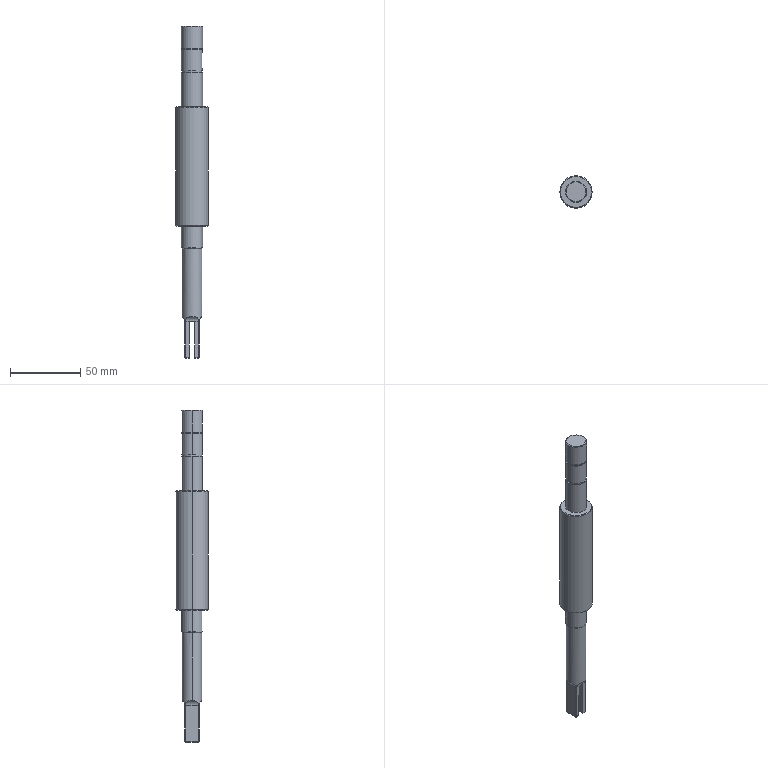Part | STEP file | Main drive shaft SGN-5-05 | 1 solid | 74 faces | box 23 x 23 x 236.35 mm | volume 57350 mm3 | cylinder 35 | plane 21 | cone 10 | spline 4 | sphere 4 | commonest cylinder face diameters 1 x10 15 x8 8 x4 13.8 x4 5 x3 3.3 x2